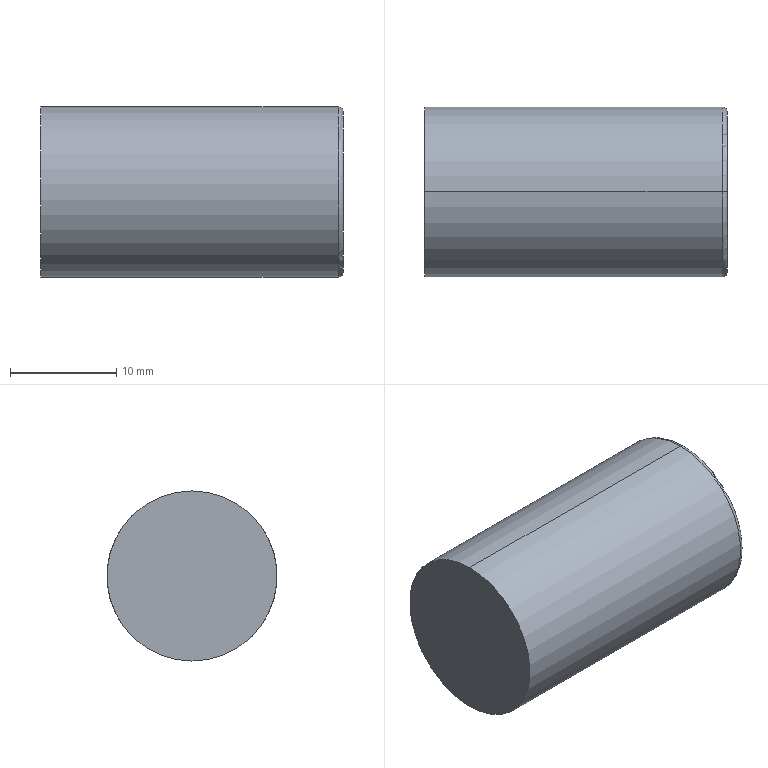Part | STEP file | 0245_Z_102_AB060-010-S1-P1_2 | 1 solid | 10 faces | box 28.5 x 16 x 16 mm | volume 5550 mm3 | cylinder 4 | cone 2 | torus 2 | plane 2 | commonest cylinder face diameters 4.2 x2 16 x2
STEP:
#1=CARTESIAN_POINT('',(0.,0.,0.));
#2=DIRECTION('',(0.,0.,1.));
#3=DIRECTION('',(1.,0.,0.));
#4=AXIS2_PLACEMENT_3D('',#1,#2,#3);
#5=CARTESIAN_POINT('',(16.1,0.,-2.1));
#6=VERTEX_POINT('',#5);
#7=CARTESIAN_POINT('',(28.5,0.,-2.1));
#8=VERTEX_POINT('',#7);
#9=CARTESIAN_POINT('',(28.5,0.,-2.1));
#10=DIRECTION('',(1.,0.,0.));
#11=VECTOR('',#10,1.);
#12=LINE('',#9,#11);
#13=CARTESIAN_POINT('',(28.5,0.,0.));
#14=DIRECTION('',(1.,0.,0.));
#15=DIRECTION('',(0.,0.,-1.));
#16=AXIS2_PLACEMENT_3D('',#13,#14,#15);
#17=CYLINDRICAL_SURFACE('',#16,2.1);
#18=CARTESIAN_POINT('',(6.283,0.));
#19=DIRECTION('',(0.,1.));
#20=VECTOR('',#19,1.);
#21=LINE('',#18,#20);
#22=(GEOMETRIC_REPRESENTATION_CONTEXT(2)PARAMETRIC_REPRESENTATION_CONTEXT()REPRESENTATION_CONTEXT('',''));
#23=DEFINITIONAL_REPRESENTATION('',(#21),#22);
#24=PCURVE('',#17,#23);
#25=CARTESIAN_POINT('',(28.5,0.,0.));
#26=DIRECTION('',(1.,0.,0.));
#27=DIRECTION('',(0.,0.,-1.));
#28=AXIS2_PLACEMENT_3D('',#25,#26,#27);
#29=CYLINDRICAL_SURFACE('',#28,2.1);
#30=CARTESIAN_POINT('',(0.,0.));
#31=DIRECTION('',(0.,1.));
#32=VECTOR('',#31,1.);
#33=LINE('',#30,#32);
#34=(GEOMETRIC_REPRESENTATION_CONTEXT(2)PARAMETRIC_REPRESENTATION_CONTEXT()REPRESENTATION_CONTEXT('',''));
#35=DEFINITIONAL_REPRESENTATION('',(#33),#34);
#36=PCURVE('',#29,#35);
#37=SURFACE_CURVE('',#12,(#24,#36),.PCURVE_S1.);
#38=EDGE_CURVE('',#6,#8,#37,.T.);
#39=ORIENTED_EDGE('',*,*,#38,.T.);
#40=CARTESIAN_POINT('',(28.5,0.,2.1));
#41=VERTEX_POINT('',#40);
#42=CARTESIAN_POINT('',(28.5,0.,0.));
#43=DIRECTION('',(1.,0.,0.));
#44=DIRECTION('',(0.,0.,-1.));
#45=AXIS2_PLACEMENT_3D('',#42,#43,#44);
#46=CIRCLE('',#45,2.1);
#47=CARTESIAN_POINT('',(0.,0.));
#48=DIRECTION('',(1.,0.));
#49=VECTOR('',#48,1.);
#50=LINE('',#47,#49);
#51=(GEOMETRIC_REPRESENTATION_CONTEXT(2)PARAMETRIC_REPRESENTATION_CONTEXT()REPRESENTATION_CONTEXT('',''));
#52=DEFINITIONAL_REPRESENTATION('',(#50),#51);
#53=PCURVE('',#17,#52);
#54=CARTESIAN_POINT('',(28.5,0.,0.));
#55=DIRECTION('',(1.,0.,0.));
#56=DIRECTION('',(0.,0.,-1.));
#57=AXIS2_PLACEMENT_3D('',#54,#55,#56);
#58=PLANE('',#57);
#59=CARTESIAN_POINT('',(0.,0.));
#60=DIRECTION('',(1.,0.));
#61=AXIS2_PLACEMENT_2D('',#59,#60);
#62=CIRCLE('',#61,2.1);
#63=(GEOMETRIC_REPRESENTATION_CONTEXT(2)PARAMETRIC_REPRESENTATION_CONTEXT()REPRESENTATION_CONTEXT('',''));
#64=DEFINITIONAL_REPRESENTATION('',(#62),#63);
#65=PCURVE('',#58,#64);
#66=SURFACE_CURVE('',#46,(#53,#65),.PCURVE_S1.);
#67=EDGE_CURVE('',#41,#8,#66,.T.);
#68=ORIENTED_EDGE('',*,*,#67,.F.);
#69=CARTESIAN_POINT('',(16.1,0.,2.1));
#70=VERTEX_POINT('',#69);
#71=CARTESIAN_POINT('',(28.5,0.,2.1));
#72=DIRECTION('',(1.,0.,0.));
#73=VECTOR('',#72,1.);
#74=LINE('',#71,#73);
#75=CARTESIAN_POINT('',(3.142,0.));
#76=DIRECTION('',(0.,1.));
#77=VECTOR('',#76,1.);
#78=LINE('',#75,#77);
#79=(GEOMETRIC_REPRESENTATION_CONTEXT(2)PARAMETRIC_REPRESENTATION_CONTEXT()REPRESENTATION_CONTEXT('',''));
#80=DEFINITIONAL_REPRESENTATION('',(#78),#79);
#81=PCURVE('',#17,#80);
#82=CARTESIAN_POINT('',(3.142,0.));
#83=DIRECTION('',(0.,1.));
#84=VECTOR('',#83,1.);
#85=LINE('',#82,#84);
#86=(GEOMETRIC_REPRESENTATION_CONTEXT(2)PARAMETRIC_REPRESENTATION_CONTEXT()REPRESENTATION_CONTEXT('',''));
#87=DEFINITIONAL_REPRESENTATION('',(#85),#86);
#88=PCURVE('',#29,#87);
#89=SURFACE_CURVE('',#74,(#81,#88),.PCURVE_S1.);
#90=EDGE_CURVE('',#70,#41,#89,.T.);
#91=ORIENTED_EDGE('',*,*,#90,.F.);
#92=CARTESIAN_POINT('',(16.1,0.,0.));
#93=DIRECTION('',(1.,0.,0.));
#94=DIRECTION('',(0.,0.,-1.));
#95=AXIS2_PLACEMENT_3D('',#92,#93,#94);
#96=CIRCLE('',#95,2.1);
#97=CARTESIAN_POINT('',(0.,-12.4));
#98=DIRECTION('',(1.,0.));
#99=VECTOR('',#98,1.);
#100=LINE('',#97,#99);
#101=(GEOMETRIC_REPRESENTATION_CONTEXT(2)PARAMETRIC_REPRESENTATION_CONTEXT()REPRESENTATION_CONTEXT('',''));
#102=DEFINITIONAL_REPRESENTATION('',(#100),#101);
#103=PCURVE('',#17,#102);
#104=CARTESIAN_POINT('',(16.1,0.,0.));
#105=DIRECTION('',(1.,0.,0.));
#106=DIRECTION('',(0.,0.,-1.));
#107=AXIS2_PLACEMENT_3D('',#104,#105,#106);
#108=CONICAL_SURFACE('',#107,2.1,1.03);
#109=CARTESIAN_POINT('',(0.,0.));
#110=DIRECTION('',(1.,0.));
#111=VECTOR('',#110,1.);
#112=LINE('',#109,#111);
#113=(GEOMETRIC_REPRESENTATION_CONTEXT(2)PARAMETRIC_REPRESENTATION_CONTEXT()REPRESENTATION_CONTEXT('',''));
#114=DEFINITIONAL_REPRESENTATION('',(#112),#113);
#115=PCURVE('',#108,#114);
#116=SURFACE_CURVE('',#96,(#103,#115),.PCURVE_S1.);
#117=EDGE_CURVE('',#70,#6,#116,.T.);
#118=ORIENTED_EDGE('',*,*,#117,.T.);
#119=EDGE_LOOP('',(#39,#68,#91,#118));
#120=FACE_BOUND('',#119,.F.);
#121=ADVANCED_FACE('',(#120),#17,.F.);
#122=ORIENTED_EDGE('',*,*,#117,.F.);
#123=CARTESIAN_POINT('',(14.838,0.,0.));
#124=VERTEX_POINT('',#123);
#125=CARTESIAN_POINT('',(16.1,0.,2.1));
#126=DIRECTION('',(0.515,0.,0.8572));
#127=VECTOR('',#126,1.);
#128=LINE('',#125,#127);
#129=CARTESIAN_POINT('',(3.142,-1.262));
#130=CARTESIAN_POINT('',(3.142,-1.243));
#131=CARTESIAN_POINT('',(3.142,-1.204));
#132=CARTESIAN_POINT('',(3.142,-1.147));
#133=CARTESIAN_POINT('',(3.142,-1.09));
#134=CARTESIAN_POINT('',(3.142,-1.032));
#135=CARTESIAN_POINT('',(3.142,-0.975));
#136=CARTESIAN_POINT('',(3.142,-0.9177));
#137=CARTESIAN_POINT('',(3.142,-0.8603));
#138=CARTESIAN_POINT('',(3.142,-0.803));
#139=CARTESIAN_POINT('',(3.142,-0.7456));
#140=CARTESIAN_POINT('',(3.142,-0.6883));
#141=CARTESIAN_POINT('',(3.142,-0.6309));
#142=CARTESIAN_POINT('',(3.142,-0.5735));
#143=CARTESIAN_POINT('',(3.142,-0.5162));
#144=CARTESIAN_POINT('',(3.142,-0.4588));
#145=CARTESIAN_POINT('',(3.142,-0.4015));
#146=CARTESIAN_POINT('',(3.142,-0.3441));
#147=CARTESIAN_POINT('',(3.142,-0.2868));
#148=CARTESIAN_POINT('',(3.142,-0.2294));
#149=CARTESIAN_POINT('',(3.142,-0.1721));
#150=CARTESIAN_POINT('',(3.142,-0.1147));
#151=CARTESIAN_POINT('',(3.142,-0.05735));
#152=CARTESIAN_POINT('',(3.142,-0.01912));
#153=CARTESIAN_POINT('',(3.142,0.));
#154=B_SPLINE_CURVE_WITH_KNOTS('',3,(#129,#130,#131,#132,#133,#134,#135,#136,#137,#138,#139,#140,#141,#142,#143,#144,#145,#146,#147,#148,#149,#150,#151,#152,#153),.UNSPECIFIED.,.F.,.F.,(4,1,1,1,1,1,1,1,1,1,1,1,1,1,1,1,1,1,1,1,1,1,4),(-2.45,-2.339,-2.227,-2.116,-2.004,-1.893,-1.782,-1.67,-1.559,-1.448,-1.336,-1.225,-1.114,-1.002,-0.8909,-0.7795,-0.6682,-0.5568,-0.4454,-0.3341,-0.2227,-0.1114,0.),.UNSPECIFIED.);
#155=(GEOMETRIC_REPRESENTATION_CONTEXT(2)PARAMETRIC_REPRESENTATION_CONTEXT()REPRESENTATION_CONTEXT('',''));
#156=DEFINITIONAL_REPRESENTATION('',(#154),#155);
#157=PCURVE('',#108,#156);
#158=CARTESIAN_POINT('',(16.1,0.,0.));
#159=DIRECTION('',(1.,0.,0.));
#160=DIRECTION('',(0.,0.,-1.));
#161=AXIS2_PLACEMENT_3D('',#158,#159,#160);
#162=CONICAL_SURFACE('',#161,2.1,1.03);
#163=CARTESIAN_POINT('',(3.142,-1.262));
#164=CARTESIAN_POINT('',(3.142,-1.243));
#165=CARTESIAN_POINT('',(3.142,-1.204));
#166=CARTESIAN_POINT('',(3.142,-1.147));
#167=CARTESIAN_POINT('',(3.142,-1.09));
#168=CARTESIAN_POINT('',(3.142,-1.032));
#169=CARTESIAN_POINT('',(3.142,-0.975));
#170=CARTESIAN_POINT('',(3.142,-0.9177));
#171=CARTESIAN_POINT('',(3.142,-0.8603));
#172=CARTESIAN_POINT('',(3.142,-0.803));
#173=CARTESIAN_POINT('',(3.142,-0.7456));
#174=CARTESIAN_POINT('',(3.142,-0.6883));
#175=CARTESIAN_POINT('',(3.142,-0.6309));
#176=CARTESIAN_POINT('',(3.142,-0.5735));
#177=CARTESIAN_POINT('',(3.142,-0.5162));
#178=CARTESIAN_POINT('',(3.142,-0.4588));
#179=CARTESIAN_POINT('',(3.142,-0.4015));
#180=CARTESIAN_POINT('',(3.142,-0.3441));
#181=CARTESIAN_POINT('',(3.142,-0.2868));
#182=CARTESIAN_POINT('',(3.142,-0.2294));
#183=CARTESIAN_POINT('',(3.142,-0.1721));
#184=CARTESIAN_POINT('',(3.142,-0.1147));
#185=CARTESIAN_POINT('',(3.142,-0.05735));
#186=CARTESIAN_POINT('',(3.142,-0.01912));
#187=CARTESIAN_POINT('',(3.142,0.));
#188=B_SPLINE_CURVE_WITH_KNOTS('',3,(#163,#164,#165,#166,#167,#168,#169,#170,#171,#172,#173,#174,#175,#176,#177,#178,#179,#180,#181,#182,#183,#184,#185,#186,#187),.UNSPECIFIED.,.F.,.F.,(4,1,1,1,1,1,1,1,1,1,1,1,1,1,1,1,1,1,1,1,1,1,4),(-2.45,-2.339,-2.227,-2.116,-2.004,-1.893,-1.782,-1.67,-1.559,-1.448,-1.336,-1.225,-1.114,-1.002,-0.8909,-0.7795,-0.6682,-0.5568,-0.4454,-0.3341,-0.2227,-0.1114,0.),.UNSPECIFIED.);
#189=(GEOMETRIC_REPRESENTATION_CONTEXT(2)PARAMETRIC_REPRESENTATION_CONTEXT()REPRESENTATION_CONTEXT('',''));
#190=DEFINITIONAL_REPRESENTATION('',(#188),#189);
#191=PCURVE('',#162,#190);
#192=SURFACE_CURVE('',#128,(#157,#191),.PCURVE_S1.);
#193=EDGE_CURVE('',#124,#70,#192,.T.);
#194=ORIENTED_EDGE('',*,*,#193,.F.);
#195=CARTESIAN_POINT('',(16.1,0.,-2.1));
#196=DIRECTION('',(0.515,0.,-0.8572));
#197=VECTOR('',#196,1.);
#198=LINE('',#195,#197);
#199=CARTESIAN_POINT('',(6.283,-1.262));
#200=CARTESIAN_POINT('',(6.283,-1.243));
#201=CARTESIAN_POINT('',(6.283,-1.204));
#202=CARTESIAN_POINT('',(6.283,-1.147));
#203=CARTESIAN_POINT('',(6.283,-1.09));
#204=CARTESIAN_POINT('',(6.283,-1.032));
#205=CARTESIAN_POINT('',(6.283,-0.975));
#206=CARTESIAN_POINT('',(6.283,-0.9177));
#207=CARTESIAN_POINT('',(6.283,-0.8603));
#208=CARTESIAN_POINT('',(6.283,-0.803));
#209=CARTESIAN_POINT('',(6.283,-0.7456));
#210=CARTESIAN_POINT('',(6.283,-0.6883));
#211=CARTESIAN_POINT('',(6.283,-0.6309));
#212=CARTESIAN_POINT('',(6.283,-0.5735));
#213=CARTESIAN_POINT('',(6.283,-0.5162));
#214=CARTESIAN_POINT('',(6.283,-0.4588));
#215=CARTESIAN_POINT('',(6.283,-0.4015));
#216=CARTESIAN_POINT('',(6.283,-0.3441));
#217=CARTESIAN_POINT('',(6.283,-0.2868));
#218=CARTESIAN_POINT('',(6.283,-0.2294));
#219=CARTESIAN_POINT('',(6.283,-0.1721));
#220=CARTESIAN_POINT('',(6.283,-0.1147));
#221=CARTESIAN_POINT('',(6.283,-0.05735));
#222=CARTESIAN_POINT('',(6.283,-0.01912));
#223=CARTESIAN_POINT('',(6.283,0.));
#224=B_SPLINE_CURVE_WITH_KNOTS('',3,(#199,#200,#201,#202,#203,#204,#205,#206,#207,#208,#209,#210,#211,#212,#213,#214,#215,#216,#217,#218,#219,#220,#221,#222,#223),.UNSPECIFIED.,.F.,.F.,(4,1,1,1,1,1,1,1,1,1,1,1,1,1,1,1,1,1,1,1,1,1,4),(-2.45,-2.339,-2.227,-2.116,-2.004,-1.893,-1.782,-1.67,-1.559,-1.448,-1.336,-1.225,-1.114,-1.002,-0.8909,-0.7795,-0.6682,-0.5568,-0.4454,-0.3341,-0.2227,-0.1114,0.),.UNSPECIFIED.);
#225=(GEOMETRIC_REPRESENTATION_CONTEXT(2)PARAMETRIC_REPRESENTATION_CONTEXT()REPRESENTATION_CONTEXT('',''));
#226=DEFINITIONAL_REPRESENTATION('',(#224),#225);
#227=PCURVE('',#108,#226);
#228=CARTESIAN_POINT('',(0.,-1.262));
#229=CARTESIAN_POINT('',(0.,-1.243));
#230=CARTESIAN_POINT('',(0.,-1.204));
#231=CARTESIAN_POINT('',(0.,-1.147));
#232=CARTESIAN_POINT('',(0.,-1.09));
#233=CARTESIAN_POINT('',(0.,-1.032));
#234=CARTESIAN_POINT('',(0.,-0.975));
#235=CARTESIAN_POINT('',(0.,-0.9177));
#236=CARTESIAN_POINT('',(0.,-0.8603));
#237=CARTESIAN_POINT('',(0.,-0.803));
#238=CARTESIAN_POINT('',(0.,-0.7456));
#239=CARTESIAN_POINT('',(0.,-0.6883));
#240=CARTESIAN_POINT('',(0.,-0.6309));
#241=CARTESIAN_POINT('',(0.,-0.5735));
#242=CARTESIAN_POINT('',(0.,-0.5162));
#243=CARTESIAN_POINT('',(0.,-0.4588));
#244=CARTESIAN_POINT('',(0.,-0.4015));
#245=CARTESIAN_POINT('',(0.,-0.3441));
#246=CARTESIAN_POINT('',(0.,-0.2868));
#247=CARTESIAN_POINT('',(0.,-0.2294));
#248=CARTESIAN_POINT('',(0.,-0.1721));
#249=CARTESIAN_POINT('',(0.,-0.1147));
#250=CARTESIAN_POINT('',(0.,-0.05735));
#251=CARTESIAN_POINT('',(0.,-0.01912));
#252=CARTESIAN_POINT('',(0.,0.));
#253=B_SPLINE_CURVE_WITH_KNOTS('',3,(#228,#229,#230,#231,#232,#233,#234,#235,#236,#237,#238,#239,#240,#241,#242,#243,#244,#245,#246,#247,#248,#249,#250,#251,#252),.UNSPECIFIED.,.F.,.F.,(4,1,1,1,1,1,1,1,1,1,1,1,1,1,1,1,1,1,1,1,1,1,4),(-2.45,-2.339,-2.227,-2.116,-2.004,-1.893,-1.782,-1.67,-1.559,-1.448,-1.336,-1.225,-1.114,-1.002,-0.8909,-0.7795,-0.6682,-0.5568,-0.4454,-0.3341,-0.2227,-0.1114,0.),.UNSPECIFIED.);
#254=(GEOMETRIC_REPRESENTATION_CONTEXT(2)PARAMETRIC_REPRESENTATION_CONTEXT()REPRESENTATION_CONTEXT('',''));
#255=DEFINITIONAL_REPRESENTATION('',(#253),#254);
#256=PCURVE('',#162,#255);
#257=SURFACE_CURVE('',#198,(#227,#256),.PCURVE_S1.);
#258=EDGE_CURVE('',#124,#6,#257,.T.);
#259=ORIENTED_EDGE('',*,*,#258,.T.);
#260=EDGE_LOOP('',(#122,#194,#259));
#261=FACE_BOUND('',#260,.F.);
#262=ADVANCED_FACE('',(#261),#108,.F.);
#263=CARTESIAN_POINT('',(28.,0.,8.));
#264=VERTEX_POINT('',#263);
#265=CARTESIAN_POINT('',(28.,0.,-8.));
#266=VERTEX_POINT('',#265);
#267=CARTESIAN_POINT('',(28.,0.,0.));
#268=DIRECTION('',(-1.,0.,0.));
#269=DIRECTION('',(0.,0.,-1.));
#270=AXIS2_PLACEMENT_3D('',#267,#268,#269);
#271=CIRCLE('',#270,8.);
#272=CARTESIAN_POINT('',(28.,0.,0.));
#273=DIRECTION('',(1.,0.,0.));
#274=DIRECTION('',(0.,0.,-1.));
#275=AXIS2_PLACEMENT_3D('',#272,#273,#274);
#276=TOROIDAL_SURFACE('',#275,7.5,0.5);
#277=CARTESIAN_POINT('',(6.283,0.));
#278=DIRECTION('',(-1.,0.));
#279=VECTOR('',#278,1.);
#280=LINE('',#277,#279);
#281=(GEOMETRIC_REPRESENTATION_CONTEXT(2)PARAMETRIC_REPRESENTATION_CONTEXT()REPRESENTATION_CONTEXT('',''));
#282=DEFINITIONAL_REPRESENTATION('',(#280),#281);
#283=PCURVE('',#276,#282);
#284=CARTESIAN_POINT('',(28.5,0.,0.));
#285=DIRECTION('',(-1.,0.,0.));
#286=DIRECTION('',(0.,0.,1.));
#287=AXIS2_PLACEMENT_3D('',#284,#285,#286);
#288=CYLINDRICAL_SURFACE('',#287,8.);
#289=CARTESIAN_POINT('',(-3.142,0.5));
#290=DIRECTION('',(1.,0.));
#291=VECTOR('',#290,1.);
#292=LINE('',#289,#291);
#293=(GEOMETRIC_REPRESENTATION_CONTEXT(2)PARAMETRIC_REPRESENTATION_CONTEXT()REPRESENTATION_CONTEXT('',''));
#294=DEFINITIONAL_REPRESENTATION('',(#292),#293);
#295=PCURVE('',#288,#294);
#296=SURFACE_CURVE('',#271,(#283,#295),.PCURVE_S1.);
#297=EDGE_CURVE('',#264,#266,#296,.T.);
#298=ORIENTED_EDGE('',*,*,#297,.F.);
#299=CARTESIAN_POINT('',(28.5,0.,7.5));
#300=VERTEX_POINT('',#299);
#301=CARTESIAN_POINT('',(28.,0.,7.5));
#302=DIRECTION('',(0.,1.,0.));
#303=DIRECTION('',(0.,0.,1.));
#304=AXIS2_PLACEMENT_3D('',#301,#302,#303);
#305=CIRCLE('',#304,0.5);
#306=CARTESIAN_POINT('',(3.142,0.));
#307=DIRECTION('',(0.,1.));
#308=VECTOR('',#307,1.);
#309=LINE('',#306,#308);
#310=(GEOMETRIC_REPRESENTATION_CONTEXT(2)PARAMETRIC_REPRESENTATION_CONTEXT()REPRESENTATION_CONTEXT('',''));
#311=DEFINITIONAL_REPRESENTATION('',(#309),#310);
#312=PCURVE('',#276,#311);
#313=CARTESIAN_POINT('',(28.,0.,0.));
#314=DIRECTION('',(1.,0.,0.));
#315=DIRECTION('',(0.,0.,-1.));
#316=AXIS2_PLACEMENT_3D('',#313,#314,#315);
#317=TOROIDAL_SURFACE('',#316,7.5,0.5);
#318=CARTESIAN_POINT('',(3.142,0.));
#319=DIRECTION('',(0.,1.));
#320=VECTOR('',#319,1.);
#321=LINE('',#318,#320);
#322=(GEOMETRIC_REPRESENTATION_CONTEXT(2)PARAMETRIC_REPRESENTATION_CONTEXT()REPRESENTATION_CONTEXT('',''));
#323=DEFINITIONAL_REPRESENTATION('',(#321),#322);
#324=PCURVE('',#317,#323);
#325=SURFACE_CURVE('',#305,(#312,#324),.PCURVE_S1.);
#326=EDGE_CURVE('',#264,#300,#325,.T.);
#327=ORIENTED_EDGE('',*,*,#326,.T.);
#328=CARTESIAN_POINT('',(28.5,0.,-7.5));
#329=VERTEX_POINT('',#328);
#330=CARTESIAN_POINT('',(28.5,0.,0.));
#331=DIRECTION('',(1.,0.,0.));
#332=DIRECTION('',(0.,0.,-1.));
#333=AXIS2_PLACEMENT_3D('',#330,#331,#332);
#334=CIRCLE('',#333,7.5);
#335=CARTESIAN_POINT('',(0.,1.571));
#336=DIRECTION('',(1.,0.));
#337=VECTOR('',#336,1.);
#338=LINE('',#335,#337);
#339=(GEOMETRIC_REPRESENTATION_CONTEXT(2)PARAMETRIC_REPRESENTATION_CONTEXT()REPRESENTATION_CONTEXT('',''));
#340=DEFINITIONAL_REPRESENTATION('',(#338),#339);
#341=PCURVE('',#276,#340);
#342=CARTESIAN_POINT('',(0.,0.));
#343=DIRECTION('',(1.,0.));
#344=AXIS2_PLACEMENT_2D('',#342,#343);
#345=CIRCLE('',#344,7.5);
#346=(GEOMETRIC_REPRESENTATION_CONTEXT(2)PARAMETRIC_REPRESENTATION_CONTEXT()REPRESENTATION_CONTEXT('',''));
#347=DEFINITIONAL_REPRESENTATION('',(#345),#346);
#348=PCURVE('',#58,#347);
#349=SURFACE_CURVE('',#334,(#341,#348),.PCURVE_S1.);
#350=EDGE_CURVE('',#329,#300,#349,.T.);
#351=ORIENTED_EDGE('',*,*,#350,.F.);
#352=CARTESIAN_POINT('',(28.,0.,-7.5));
#353=DIRECTION('',(0.,-1.,0.));
#354=DIRECTION('',(0.,0.,-1.));
#355=AXIS2_PLACEMENT_3D('',#352,#353,#354);
#356=CIRCLE('',#355,0.5);
#357=CARTESIAN_POINT('',(0.,0.));
#358=DIRECTION('',(0.,1.));
#359=VECTOR('',#358,1.);
#360=LINE('',#357,#359);
#361=(GEOMETRIC_REPRESENTATION_CONTEXT(2)PARAMETRIC_REPRESENTATION_CONTEXT()REPRESENTATION_CONTEXT('',''));
#362=DEFINITIONAL_REPRESENTATION('',(#360),#361);
#363=PCURVE('',#276,#362);
#364=CARTESIAN_POINT('',(6.283,0.));
#365=DIRECTION('',(0.,1.));
#366=VECTOR('',#365,1.);
#367=LINE('',#364,#366);
#368=(GEOMETRIC_REPRESENTATION_CONTEXT(2)PARAMETRIC_REPRESENTATION_CONTEXT()REPRESENTATION_CONTEXT('',''));
#369=DEFINITIONAL_REPRESENTATION('',(#367),#368);
#370=PCURVE('',#317,#369);
#371=SURFACE_CURVE('',#356,(#363,#370),.PCURVE_S1.);
#372=EDGE_CURVE('',#266,#329,#371,.T.);
#373=ORIENTED_EDGE('',*,*,#372,.F.);
#374=EDGE_LOOP('',(#298,#327,#351,#373));
#375=FACE_BOUND('',#374,.T.);
#376=ADVANCED_FACE('',(#375),#276,.T.);
#377=ORIENTED_EDGE('',*,*,#297,.T.);
#378=CARTESIAN_POINT('',(0.,0.,-8.));
#379=VERTEX_POINT('',#378);
#380=CARTESIAN_POINT('',(28.5,0.,-8.));
#381=DIRECTION('',(-1.,0.,0.));
#382=VECTOR('',#381,1.);
#383=LINE('',#380,#382);
#384=CARTESIAN_POINT('',(3.142,0.));
#385=DIRECTION('',(0.,1.));
#386=VECTOR('',#385,1.);
#387=LINE('',#384,#386);
#388=(GEOMETRIC_REPRESENTATION_CONTEXT(2)PARAMETRIC_REPRESENTATION_CONTEXT()REPRESENTATION_CONTEXT('',''));
#389=DEFINITIONAL_REPRESENTATION('',(#387),#388);
#390=PCURVE('',#288,#389);
#391=CARTESIAN_POINT('',(28.5,0.,0.));
#392=DIRECTION('',(-1.,0.,0.));
#393=DIRECTION('',(0.,0.,1.));
#394=AXIS2_PLACEMENT_3D('',#391,#392,#393);
#395=CYLINDRICAL_SURFACE('',#394,8.);
#396=CARTESIAN_POINT('',(3.142,0.));
#397=DIRECTION('',(0.,1.));
#398=VECTOR('',#397,1.);
#399=LINE('',#396,#398);
#400=(GEOMETRIC_REPRESENTATION_CONTEXT(2)PARAMETRIC_REPRESENTATION_CONTEXT()REPRESENTATION_CONTEXT('',''));
#401=DEFINITIONAL_REPRESENTATION('',(#399),#400);
#402=PCURVE('',#395,#401);
#403=SURFACE_CURVE('',#383,(#390,#402),.PCURVE_S1.);
#404=EDGE_CURVE('',#266,#379,#403,.T.);
#405=ORIENTED_EDGE('',*,*,#404,.T.);
#406=CARTESIAN_POINT('',(0.,0.,8.));
#407=VERTEX_POINT('',#406);
#408=CARTESIAN_POINT('',(0.,0.,0.));
#409=DIRECTION('',(1.,0.,0.));
#410=DIRECTION('',(0.,0.,-1.));
#411=AXIS2_PLACEMENT_3D('',#408,#409,#410);
#412=CIRCLE('',#411,8.);
#413=CARTESIAN_POINT('',(3.142,28.5));
#414=DIRECTION('',(-1.,0.));
#415=VECTOR('',#414,1.);
#416=LINE('',#413,#415);
#417=(GEOMETRIC_REPRESENTATION_CONTEXT(2)PARAMETRIC_REPRESENTATION_CONTEXT()REPRESENTATION_CONTEXT('',''));
#418=DEFINITIONAL_REPRESENTATION('',(#416),#417);
#419=PCURVE('',#288,#418);
#420=CARTESIAN_POINT('',(0.,0.,0.));
#421=DIRECTION('',(1.,0.,0.));
#422=DIRECTION('',(0.,0.,-1.));
#423=AXIS2_PLACEMENT_3D('',#420,#421,#422);
#424=PLANE('',#423);
#425=CARTESIAN_POINT('',(0.,0.));
#426=DIRECTION('',(1.,0.));
#427=AXIS2_PLACEMENT_2D('',#425,#426);
#428=CIRCLE('',#427,8.);
#429=(GEOMETRIC_REPRESENTATION_CONTEXT(2)PARAMETRIC_REPRESENTATION_CONTEXT()REPRESENTATION_CONTEXT('',''));
#430=DEFINITIONAL_REPRESENTATION('',(#428),#429);
#431=PCURVE('',#424,#430);
#432=SURFACE_CURVE('',#412,(#419,#431),.PCURVE_S1.);
#433=EDGE_CURVE('',#379,#407,#432,.T.);
#434=ORIENTED_EDGE('',*,*,#433,.T.);
#435=CARTESIAN_POINT('',(28.5,0.,8.));
#436=DIRECTION('',(-1.,0.,0.));
#437=VECTOR('',#436,1.);
#438=LINE('',#435,#437);
#439=CARTESIAN_POINT('',(0.,0.));
#440=DIRECTION('',(0.,1.));
#441=VECTOR('',#440,1.);
#442=LINE('',#439,#441);
#443=(GEOMETRIC_REPRESENTATION_CONTEXT(2)PARAMETRIC_REPRESENTATION_CONTEXT()REPRESENTATION_CONTEXT('',''));
#444=DEFINITIONAL_REPRESENTATION('',(#442),#443);
#445=PCURVE('',#288,#444);
#446=CARTESIAN_POINT('',(6.283,0.));
#447=DIRECTION('',(0.,1.));
#448=VECTOR('',#447,1.);
#449=LINE('',#446,#448);
#450=(GEOMETRIC_REPRESENTATION_CONTEXT(2)PARAMETRIC_REPRESENTATION_CONTEXT()REPRESENTATION_CONTEXT('',''));
#451=DEFINITIONAL_REPRESENTATION('',(#449),#450);
#452=PCURVE('',#395,#451);
#453=SURFACE_CURVE('',#438,(#445,#452),.PCURVE_S1.);
#454=EDGE_CURVE('',#264,#407,#453,.T.);
#455=ORIENTED_EDGE('',*,*,#454,.F.);
#456=EDGE_LOOP('',(#377,#405,#434,#455));
#457=FACE_BOUND('',#456,.T.);
#458=ADVANCED_FACE('',(#457),#288,.T.);
#459=ORIENTED_EDGE('',*,*,#404,.F.);
#460=CARTESIAN_POINT('',(28.,0.,0.));
#461=DIRECTION('',(-1.,0.,0.));
#462=DIRECTION('',(0.,0.,-1.));
#463=AXIS2_PLACEMENT_3D('',#460,#461,#462);
#464=CIRCLE('',#463,8.);
#465=CARTESIAN_POINT('',(3.142,0.5));
#466=DIRECTION('',(1.,0.));
#467=VECTOR('',#466,1.);
#468=LINE('',#465,#467);
#469=(GEOMETRIC_REPRESENTATION_CONTEXT(2)PARAMETRIC_REPRESENTATION_CONTEXT()REPRESENTATION_CONTEXT('',''));
#470=DEFINITIONAL_REPRESENTATION('',(#468),#469);
#471=PCURVE('',#395,#470);
#472=CARTESIAN_POINT('',(6.283,0.));
#473=DIRECTION('',(-1.,0.));
#474=VECTOR('',#473,1.);
#475=LINE('',#472,#474);
#476=(GEOMETRIC_REPRESENTATION_CONTEXT(2)PARAMETRIC_REPRESENTATION_CONTEXT()REPRESENTATION_CONTEXT('',''));
#477=DEFINITIONAL_REPRESENTATION('',(#475),#476);
#478=PCURVE('',#317,#477);
#479=SURFACE_CURVE('',#464,(#471,#478),.PCURVE_S1.);
#480=EDGE_CURVE('',#266,#264,#479,.T.);
#481=ORIENTED_EDGE('',*,*,#480,.T.);
#482=ORIENTED_EDGE('',*,*,#454,.T.);
#483=CARTESIAN_POINT('',(0.,0.,0.));
#484=DIRECTION('',(1.,0.,0.));
#485=DIRECTION('',(0.,0.,-1.));
#486=AXIS2_PLACEMENT_3D('',#483,#484,#485);
#487=CIRCLE('',#486,8.);
#488=CARTESIAN_POINT('',(9.425,28.5));
#489=DIRECTION('',(-1.,0.));
#490=VECTOR('',#489,1.);
#491=LINE('',#488,#490);
#492=(GEOMETRIC_REPRESENTATION_CONTEXT(2)PARAMETRIC_REPRESENTATION_CONTEXT()REPRESENTATION_CONTEXT('',''));
#493=DEFINITIONAL_REPRESENTATION('',(#491),#492);
#494=PCURVE('',#395,#493);
#495=CARTESIAN_POINT('',(0.,0.));
#496=DIRECTION('',(1.,0.));
#497=AXIS2_PLACEMENT_2D('',#495,#496);
#498=CIRCLE('',#497,8.);
#499=(GEOMETRIC_REPRESENTATION_CONTEXT(2)PARAMETRIC_REPRESENTATION_CONTEXT()REPRESENTATION_CONTEXT('',''));
#500=DEFINITIONAL_REPRESENTATION('',(#498),#499);
#501=PCURVE('',#424,#500);
#502=SURFACE_CURVE('',#487,(#494,#501),.PCURVE_S1.);
#503=EDGE_CURVE('',#407,#379,#502,.T.);
#504=ORIENTED_EDGE('',*,*,#503,.T.);
#505=EDGE_LOOP('',(#459,#481,#482,#504));
#506=FACE_BOUND('',#505,.T.);
#507=ADVANCED_FACE('',(#506),#395,.T.);
#508=CARTESIAN_POINT('',(28.5,0.,0.));
#509=DIRECTION('',(1.,0.,0.));
#510=DIRECTION('',(0.,0.,-1.));
#511=AXIS2_PLACEMENT_3D('',#508,#509,#510);
#512=CIRCLE('',#511,2.1);
#513=CARTESIAN_POINT('',(0.,0.));
#514=DIRECTION('',(1.,0.));
#515=AXIS2_PLACEMENT_2D('',#513,#514);
#516=CIRCLE('',#515,2.1);
#517=(GEOMETRIC_REPRESENTATION_CONTEXT(2)PARAMETRIC_REPRESENTATION_CONTEXT()REPRESENTATION_CONTEXT('',''));
#518=DEFINITIONAL_REPRESENTATION('',(#516),#517);
#519=PCURVE('',#58,#518);
#520=CARTESIAN_POINT('',(0.,0.));
#521=DIRECTION('',(1.,0.));
#522=VECTOR('',#521,1.);
#523=LINE('',#520,#522);
#524=(GEOMETRIC_REPRESENTATION_CONTEXT(2)PARAMETRIC_REPRESENTATION_CONTEXT()REPRESENTATION_CONTEXT('',''));
#525=DEFINITIONAL_REPRESENTATION('',(#523),#524);
#526=PCURVE('',#29,#525);
#527=SURFACE_CURVE('',#512,(#519,#526),.PCURVE_S1.);
#528=EDGE_CURVE('',#8,#41,#527,.T.);
#529=ORIENTED_EDGE('',*,*,#528,.F.);
#530=ORIENTED_EDGE('',*,*,#67,.F.);
#531=EDGE_LOOP('',(#529,#530));
#532=FACE_BOUND('',#531,.T.);
#533=ORIENTED_EDGE('',*,*,#350,.T.);
#534=CARTESIAN_POINT('',(28.5,0.,0.));
#535=DIRECTION('',(1.,0.,0.));
#536=DIRECTION('',(0.,0.,-1.));
#537=AXIS2_PLACEMENT_3D('',#534,#535,#536);
#538=CIRCLE('',#537,7.5);
#539=CARTESIAN_POINT('',(0.,0.));
#540=DIRECTION('',(1.,0.));
#541=AXIS2_PLACEMENT_2D('',#539,#540);
#542=CIRCLE('',#541,7.5);
#543=(GEOMETRIC_REPRESENTATION_CONTEXT(2)PARAMETRIC_REPRESENTATION_CONTEXT()REPRESENTATION_CONTEXT('',''));
#544=DEFINITIONAL_REPRESENTATION('',(#542),#543);
#545=PCURVE('',#58,#544);
#546=CARTESIAN_POINT('',(0.,1.571));
#547=DIRECTION('',(1.,0.));
#548=VECTOR('',#547,1.);
#549=LINE('',#546,#548);
#550=(GEOMETRIC_REPRESENTATION_CONTEXT(2)PARAMETRIC_REPRESENTATION_CONTEXT()REPRESENTATION_CONTEXT('',''));
#551=DEFINITIONAL_REPRESENTATION('',(#549),#550);
#552=PCURVE('',#317,#551);
#553=SURFACE_CURVE('',#538,(#545,#552),.PCURVE_S1.);
#554=EDGE_CURVE('',#300,#329,#553,.T.);
#555=ORIENTED_EDGE('',*,*,#554,.T.);
#556=EDGE_LOOP('',(#533,#555));
#557=FACE_BOUND('',#556,.T.);
#558=ADVANCED_FACE('',(#532,#557),#58,.T.);
#559=ORIENTED_EDGE('',*,*,#503,.F.);
#560=ORIENTED_EDGE('',*,*,#433,.F.);
#561=EDGE_LOOP('',(#559,#560));
#562=FACE_BOUND('',#561,.T.);
#563=ADVANCED_FACE('',(#562),#424,.F.);
#564=ORIENTED_EDGE('',*,*,#326,.F.);
#565=ORIENTED_EDGE('',*,*,#480,.F.);
#566=ORIENTED_EDGE('',*,*,#372,.T.);
#567=ORIENTED_EDGE('',*,*,#554,.F.);
#568=EDGE_LOOP('',(#564,#565,#566,#567));
#569=FACE_BOUND('',#568,.T.);
#570=ADVANCED_FACE('',(#569),#317,.T.);
#571=CARTESIAN_POINT('',(16.1,0.,0.));
#572=DIRECTION('',(1.,0.,0.));
#573=DIRECTION('',(0.,0.,-1.));
#574=AXIS2_PLACEMENT_3D('',#571,#572,#573);
#575=CIRCLE('',#574,2.1);
#576=CARTESIAN_POINT('',(0.,0.));
#577=DIRECTION('',(1.,0.));
#578=VECTOR('',#577,1.);
#579=LINE('',#576,#578);
#580=(GEOMETRIC_REPRESENTATION_CONTEXT(2)PARAMETRIC_REPRESENTATION_CONTEXT()REPRESENTATION_CONTEXT('',''));
#581=DEFINITIONAL_REPRESENTATION('',(#579),#580);
#582=PCURVE('',#162,#581);
#583=CARTESIAN_POINT('',(0.,-12.4));
#584=DIRECTION('',(1.,0.));
#585=VECTOR('',#584,1.);
#586=LINE('',#583,#585);
#587=(GEOMETRIC_REPRESENTATION_CONTEXT(2)PARAMETRIC_REPRESENTATION_CONTEXT()REPRESENTATION_CONTEXT('',''));
#588=DEFINITIONAL_REPRESENTATION('',(#586),#587);
#589=PCURVE('',#29,#588);
#590=SURFACE_CURVE('',#575,(#582,#589),.PCURVE_S1.);
#591=EDGE_CURVE('',#6,#70,#590,.T.);
#592=ORIENTED_EDGE('',*,*,#591,.F.);
#593=ORIENTED_EDGE('',*,*,#258,.F.);
#594=ORIENTED_EDGE('',*,*,#193,.T.);
#595=EDGE_LOOP('',(#592,#593,#594));
#596=FACE_BOUND('',#595,.F.);
#597=ADVANCED_FACE('',(#596),#162,.F.);
#598=ORIENTED_EDGE('',*,*,#528,.F.);
#599=ORIENTED_EDGE('',*,*,#38,.F.);
#600=ORIENTED_EDGE('',*,*,#591,.T.);
#601=ORIENTED_EDGE('',*,*,#90,.T.);
#602=EDGE_LOOP('',(#598,#599,#600,#601));
#603=FACE_BOUND('',#602,.F.);
#604=ADVANCED_FACE('',(#603),#29,.F.);
#605=CLOSED_SHELL('',(#121,#262,#376,#458,#507,#558,#563,#570,#597,#604));
#606=MANIFOLD_SOLID_BREP('',#605);
#607=(LENGTH_UNIT()NAMED_UNIT(*)SI_UNIT(.MILLI.,.METRE.));
#608=UNCERTAINTY_MEASURE_WITH_UNIT(LENGTH_MEASURE(0.0000001),#607,'','');
#609=(NAMED_UNIT(*)PLANE_ANGLE_UNIT()SI_UNIT($,.RADIAN.));
#610=(NAMED_UNIT(*)SI_UNIT($,.STERADIAN.)SOLID_ANGLE_UNIT());
#611=(GEOMETRIC_REPRESENTATION_CONTEXT(3)GLOBAL_UNCERTAINTY_ASSIGNED_CONTEXT((#608))GLOBAL_UNIT_ASSIGNED_CONTEXT((#607,#609,#610))REPRESENTATION_CONTEXT('',''));
#612=ADVANCED_BREP_SHAPE_REPRESENTATION('',(#4,#606),#611);